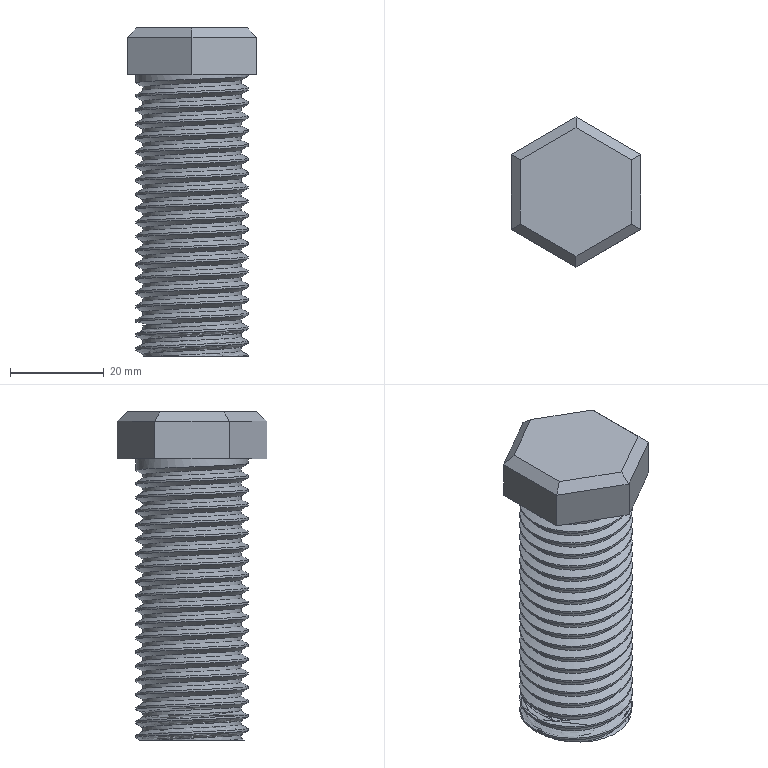Part | NX | features DATUM_CSYS 3, EXTRUDE 2, SKETCH 2, CHAMFER 1, THREADS 1 | 1 solid | 21 faces | box 27.713 x 32 x 70 mm | volume 30636 mm3 | plane 16 | spline 3 | cylinder 2 | commonest cylinder face diameters 21 x1 24 x1